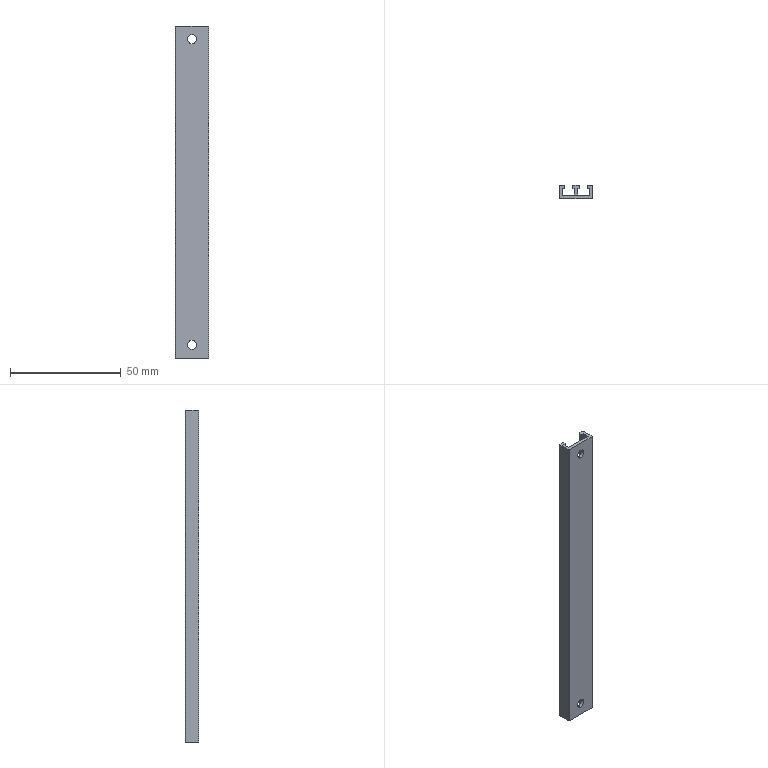Part | STEP file | 06-04 sensor mounting strip | 1 solid | 39 faces | box 15 x 6 x 150 mm | volume 6689 mm3 | plane 23 | cylinder 16 | commonest cylinder face diameters 0.4 x12 4 x4
STEP:
#1=CARTESIAN_POINT('',(7.5,0.,-146.));
#2=VERTEX_POINT('',#1);
#3=CARTESIAN_POINT('',(7.5,0.,-142.));
#4=VERTEX_POINT('',#3);
#5=CARTESIAN_POINT('',(7.5,0.,-144.));
#6=DIRECTION('',(0.,1.,0.));
#7=DIRECTION('',(0.,0.,-1.));
#8=AXIS2_PLACEMENT_3D('',#5,#6,#7);
#9=CIRCLE('',#8,2.);
#10=EDGE_CURVE('',#2,#4,#9,.T.);
#11=ORIENTED_EDGE('',*,*,#10,.F.);
#12=CARTESIAN_POINT('',(7.5,1.5,-146.));
#13=VERTEX_POINT('',#12);
#14=CARTESIAN_POINT('',(7.5,0.,-146.));
#15=DIRECTION('',(0.,1.,0.));
#16=VECTOR('',#15,1000.);
#17=LINE('',#14,#16);
#18=EDGE_CURVE('',#2,#13,#17,.T.);
#19=ORIENTED_EDGE('',*,*,#18,.T.);
#20=CARTESIAN_POINT('',(7.5,1.5,-142.));
#21=VERTEX_POINT('',#20);
#22=CARTESIAN_POINT('',(7.5,1.5,-144.));
#23=DIRECTION('',(0.,1.,0.));
#24=DIRECTION('',(0.,0.,-1.));
#25=AXIS2_PLACEMENT_3D('',#22,#23,#24);
#26=CIRCLE('',#25,2.);
#27=EDGE_CURVE('',#13,#21,#26,.T.);
#28=ORIENTED_EDGE('',*,*,#27,.T.);
#29=CARTESIAN_POINT('',(7.5,0.,-142.));
#30=DIRECTION('',(0.,1.,0.));
#31=VECTOR('',#30,1000.);
#32=LINE('',#29,#31);
#33=EDGE_CURVE('',#4,#21,#32,.T.);
#34=ORIENTED_EDGE('',*,*,#33,.F.);
#35=EDGE_LOOP('',(#11,#19,#28,#34));
#36=FACE_OUTER_BOUND('',#35,.T.);
#37=CARTESIAN_POINT('',(7.5,0.,-144.));
#38=DIRECTION('',(0.,1.,0.));
#39=DIRECTION('',(0.,0.,1.));
#40=AXIS2_PLACEMENT_3D('',#37,#38,#39);
#41=CYLINDRICAL_SURFACE('',#40,2.);
#42=ADVANCED_FACE('',(#36),#41,.F.);
#43=CARTESIAN_POINT('',(7.5,0.,-8.));
#44=VERTEX_POINT('',#43);
#45=CARTESIAN_POINT('',(7.5,0.,-4.));
#46=VERTEX_POINT('',#45);
#47=CARTESIAN_POINT('',(7.5,0.,-6.));
#48=DIRECTION('',(0.,1.,0.));
#49=DIRECTION('',(0.,0.,1.));
#50=AXIS2_PLACEMENT_3D('',#47,#48,#49);
#51=CIRCLE('',#50,2.);
#52=EDGE_CURVE('',#44,#46,#51,.T.);
#53=ORIENTED_EDGE('',*,*,#52,.F.);
#54=CARTESIAN_POINT('',(7.5,1.5,-8.));
#55=VERTEX_POINT('',#54);
#56=CARTESIAN_POINT('',(7.5,0.,-8.));
#57=DIRECTION('',(0.,1.,0.));
#58=VECTOR('',#57,1000.);
#59=LINE('',#56,#58);
#60=EDGE_CURVE('',#44,#55,#59,.T.);
#61=ORIENTED_EDGE('',*,*,#60,.T.);
#62=CARTESIAN_POINT('',(7.5,1.5,-4.));
#63=VERTEX_POINT('',#62);
#64=CARTESIAN_POINT('',(7.5,1.5,-6.));
#65=DIRECTION('',(0.,1.,0.));
#66=DIRECTION('',(0.,0.,1.));
#67=AXIS2_PLACEMENT_3D('',#64,#65,#66);
#68=CIRCLE('',#67,2.);
#69=EDGE_CURVE('',#55,#63,#68,.T.);
#70=ORIENTED_EDGE('',*,*,#69,.T.);
#71=CARTESIAN_POINT('',(7.5,0.,-4.));
#72=DIRECTION('',(0.,1.,0.));
#73=VECTOR('',#72,1000.);
#74=LINE('',#71,#73);
#75=EDGE_CURVE('',#46,#63,#74,.T.);
#76=ORIENTED_EDGE('',*,*,#75,.F.);
#77=EDGE_LOOP('',(#53,#61,#70,#76));
#78=FACE_OUTER_BOUND('',#77,.T.);
#79=CARTESIAN_POINT('',(7.5,0.,-6.));
#80=DIRECTION('',(0.,1.,0.));
#81=DIRECTION('',(0.,0.,1.));
#82=AXIS2_PLACEMENT_3D('',#79,#80,#81);
#83=CYLINDRICAL_SURFACE('',#82,2.);
#84=ADVANCED_FACE('',(#78),#83,.F.);
#85=CARTESIAN_POINT('',(1.25,1.5,-150.));
#86=VERTEX_POINT('',#85);
#87=CARTESIAN_POINT('',(1.25,4.5,-150.));
#88=VERTEX_POINT('',#87);
#89=CARTESIAN_POINT('',(1.25,4.5,-150.));
#90=DIRECTION('',(0.,1.,0.));
#91=VECTOR('',#90,1000.);
#92=LINE('',#89,#91);
#93=EDGE_CURVE('',#86,#88,#92,.T.);
#94=ORIENTED_EDGE('',*,*,#93,.F.);
#95=CARTESIAN_POINT('',(13.75,1.5,-150.));
#96=VERTEX_POINT('',#95);
#97=CARTESIAN_POINT('',(8.25,1.5,-150.));
#98=DIRECTION('',(-1.,0.,0.));
#99=VECTOR('',#98,1000.);
#100=LINE('',#97,#99);
#101=EDGE_CURVE('',#96,#86,#100,.T.);
#102=ORIENTED_EDGE('',*,*,#101,.F.);
#103=CARTESIAN_POINT('',(13.75,4.5,-150.));
#104=VERTEX_POINT('',#103);
#105=CARTESIAN_POINT('',(13.75,4.5,-150.));
#106=DIRECTION('',(0.,-1.,0.));
#107=VECTOR('',#106,1000.);
#108=LINE('',#105,#107);
#109=EDGE_CURVE('',#104,#96,#108,.T.);
#110=ORIENTED_EDGE('',*,*,#109,.F.);
#111=CARTESIAN_POINT('',(12.95,4.5,-150.));
#112=VERTEX_POINT('',#111);
#113=CARTESIAN_POINT('',(12.75,4.5,-150.));
#114=DIRECTION('',(1.,0.,0.));
#115=VECTOR('',#114,1000.);
#116=LINE('',#113,#115);
#117=EDGE_CURVE('',#112,#104,#116,.T.);
#118=ORIENTED_EDGE('',*,*,#117,.F.);
#119=CARTESIAN_POINT('',(12.75,4.7,-150.));
#120=VERTEX_POINT('',#119);
#121=CARTESIAN_POINT('',(12.95,4.7,-150.));
#122=DIRECTION('',(0.,0.,-1.));
#123=DIRECTION('',(1.,0.,0.));
#124=AXIS2_PLACEMENT_3D('',#121,#122,#123);
#125=CIRCLE('',#124,0.2);
#126=EDGE_CURVE('',#112,#120,#125,.T.);
#127=ORIENTED_EDGE('',*,*,#126,.T.);
#128=CARTESIAN_POINT('',(12.75,5.8,-150.));
#129=VERTEX_POINT('',#128);
#130=CARTESIAN_POINT('',(12.75,6.,-150.));
#131=DIRECTION('',(0.,-1.,0.));
#132=VECTOR('',#131,1000.);
#133=LINE('',#130,#132);
#134=EDGE_CURVE('',#129,#120,#133,.T.);
#135=ORIENTED_EDGE('',*,*,#134,.F.);
#136=CARTESIAN_POINT('',(12.95,6.,-150.));
#137=VERTEX_POINT('',#136);
#138=CARTESIAN_POINT('',(12.95,5.8,-150.));
#139=DIRECTION('',(0.,0.,-1.));
#140=DIRECTION('',(1.,0.,0.));
#141=AXIS2_PLACEMENT_3D('',#138,#139,#140);
#142=CIRCLE('',#141,0.2);
#143=EDGE_CURVE('',#129,#137,#142,.T.);
#144=ORIENTED_EDGE('',*,*,#143,.T.);
#145=CARTESIAN_POINT('',(14.8,6.,-150.));
#146=VERTEX_POINT('',#145);
#147=CARTESIAN_POINT('',(15.,6.,-150.));
#148=DIRECTION('',(-1.,0.,0.));
#149=VECTOR('',#148,1000.);
#150=LINE('',#147,#149);
#151=EDGE_CURVE('',#146,#137,#150,.T.);
#152=ORIENTED_EDGE('',*,*,#151,.F.);
#153=CARTESIAN_POINT('',(15.,5.8,-150.));
#154=VERTEX_POINT('',#153);
#155=CARTESIAN_POINT('',(14.8,5.8,-150.));
#156=DIRECTION('',(0.,0.,-1.));
#157=DIRECTION('',(1.,0.,0.));
#158=AXIS2_PLACEMENT_3D('',#155,#156,#157);
#159=CIRCLE('',#158,0.2);
#160=EDGE_CURVE('',#146,#154,#159,.T.);
#161=ORIENTED_EDGE('',*,*,#160,.T.);
#162=CARTESIAN_POINT('',(15.,0.2,-150.));
#163=VERTEX_POINT('',#162);
#164=CARTESIAN_POINT('',(15.,6.,-150.));
#165=DIRECTION('',(0.,1.,0.));
#166=VECTOR('',#165,1000.);
#167=LINE('',#164,#166);
#168=EDGE_CURVE('',#163,#154,#167,.T.);
#169=ORIENTED_EDGE('',*,*,#168,.F.);
#170=CARTESIAN_POINT('',(14.8,0.,-150.));
#171=VERTEX_POINT('',#170);
#172=CARTESIAN_POINT('',(14.8,0.2,-150.));
#173=DIRECTION('',(0.,0.,-1.));
#174=DIRECTION('',(1.,0.,0.));
#175=AXIS2_PLACEMENT_3D('',#172,#173,#174);
#176=CIRCLE('',#175,0.2);
#177=EDGE_CURVE('',#163,#171,#176,.T.);
#178=ORIENTED_EDGE('',*,*,#177,.T.);
#179=CARTESIAN_POINT('',(0.2,0.,-150.));
#180=VERTEX_POINT('',#179);
#181=CARTESIAN_POINT('',(0.,0.,-150.));
#182=DIRECTION('',(1.,0.,0.));
#183=VECTOR('',#182,1000.);
#184=LINE('',#181,#183);
#185=EDGE_CURVE('',#180,#171,#184,.T.);
#186=ORIENTED_EDGE('',*,*,#185,.F.);
#187=CARTESIAN_POINT('',(0.,0.2,-150.));
#188=VERTEX_POINT('',#187);
#189=CARTESIAN_POINT('',(0.2,0.2,-150.));
#190=DIRECTION('',(0.,0.,-1.));
#191=DIRECTION('',(1.,0.,0.));
#192=AXIS2_PLACEMENT_3D('',#189,#190,#191);
#193=CIRCLE('',#192,0.2);
#194=EDGE_CURVE('',#180,#188,#193,.T.);
#195=ORIENTED_EDGE('',*,*,#194,.T.);
#196=CARTESIAN_POINT('',(0.,5.8,-150.));
#197=VERTEX_POINT('',#196);
#198=CARTESIAN_POINT('',(0.,6.,-150.));
#199=DIRECTION('',(0.,-1.,0.));
#200=VECTOR('',#199,1000.);
#201=LINE('',#198,#200);
#202=EDGE_CURVE('',#197,#188,#201,.T.);
#203=ORIENTED_EDGE('',*,*,#202,.F.);
#204=CARTESIAN_POINT('',(0.2,6.,-150.));
#205=VERTEX_POINT('',#204);
#206=CARTESIAN_POINT('',(0.2,5.8,-150.));
#207=DIRECTION('',(0.,0.,-1.));
#208=DIRECTION('',(1.,0.,0.));
#209=AXIS2_PLACEMENT_3D('',#206,#207,#208);
#210=CIRCLE('',#209,0.2);
#211=EDGE_CURVE('',#197,#205,#210,.T.);
#212=ORIENTED_EDGE('',*,*,#211,.T.);
#213=CARTESIAN_POINT('',(2.05,6.,-150.));
#214=VERTEX_POINT('',#213);
#215=CARTESIAN_POINT('',(2.25,6.,-150.));
#216=DIRECTION('',(-1.,0.,0.));
#217=VECTOR('',#216,1000.);
#218=LINE('',#215,#217);
#219=EDGE_CURVE('',#214,#205,#218,.T.);
#220=ORIENTED_EDGE('',*,*,#219,.F.);
#221=CARTESIAN_POINT('',(2.25,5.8,-150.));
#222=VERTEX_POINT('',#221);
#223=CARTESIAN_POINT('',(2.05,5.8,-150.));
#224=DIRECTION('',(0.,0.,-1.));
#225=DIRECTION('',(1.,0.,0.));
#226=AXIS2_PLACEMENT_3D('',#223,#224,#225);
#227=CIRCLE('',#226,0.2);
#228=EDGE_CURVE('',#214,#222,#227,.T.);
#229=ORIENTED_EDGE('',*,*,#228,.T.);
#230=CARTESIAN_POINT('',(2.25,4.7,-150.));
#231=VERTEX_POINT('',#230);
#232=CARTESIAN_POINT('',(2.25,6.,-150.));
#233=DIRECTION('',(0.,1.,0.));
#234=VECTOR('',#233,1000.);
#235=LINE('',#232,#234);
#236=EDGE_CURVE('',#231,#222,#235,.T.);
#237=ORIENTED_EDGE('',*,*,#236,.F.);
#238=CARTESIAN_POINT('',(2.05,4.5,-150.));
#239=VERTEX_POINT('',#238);
#240=CARTESIAN_POINT('',(2.05,4.7,-150.));
#241=DIRECTION('',(0.,0.,-1.));
#242=DIRECTION('',(1.,0.,0.));
#243=AXIS2_PLACEMENT_3D('',#240,#241,#242);
#244=CIRCLE('',#243,0.2);
#245=EDGE_CURVE('',#231,#239,#244,.T.);
#246=ORIENTED_EDGE('',*,*,#245,.T.);
#247=CARTESIAN_POINT('',(1.25,4.5,-150.));
#248=DIRECTION('',(1.,0.,0.));
#249=VECTOR('',#248,1000.);
#250=LINE('',#247,#249);
#251=EDGE_CURVE('',#88,#239,#250,.T.);
#252=ORIENTED_EDGE('',*,*,#251,.F.);
#253=EDGE_LOOP('',(#94,#102,#110,#118,#127,#135,#144,#152,#161,#169,#178,#186,#195,#203,#212,#220,#229,#237,#246,#252));
#254=FACE_OUTER_BOUND('',#253,.T.);
#255=CARTESIAN_POINT('',(0.,0.,-150.));
#256=DIRECTION('',(0.,0.,1.));
#257=DIRECTION('',(1.,0.,0.));
#258=AXIS2_PLACEMENT_3D('',#255,#256,#257);
#259=PLANE('',#258);
#260=ADVANCED_FACE('',(#254),#259,.F.);
#261=CARTESIAN_POINT('',(13.75,4.5,0.));
#262=VERTEX_POINT('',#261);
#263=CARTESIAN_POINT('',(13.75,1.5,0.));
#264=VERTEX_POINT('',#263);
#265=CARTESIAN_POINT('',(13.75,4.5,0.));
#266=DIRECTION('',(0.,-1.,0.));
#267=VECTOR('',#266,1000.);
#268=LINE('',#265,#267);
#269=EDGE_CURVE('',#262,#264,#268,.T.);
#270=ORIENTED_EDGE('',*,*,#269,.T.);
#271=CARTESIAN_POINT('',(1.25,1.5,0.));
#272=VERTEX_POINT('',#271);
#273=CARTESIAN_POINT('',(1.25,1.5,0.));
#274=DIRECTION('',(-1.,0.,0.));
#275=VECTOR('',#274,1000.);
#276=LINE('',#273,#275);
#277=EDGE_CURVE('',#264,#272,#276,.T.);
#278=ORIENTED_EDGE('',*,*,#277,.T.);
#279=CARTESIAN_POINT('',(1.25,4.5,0.));
#280=VERTEX_POINT('',#279);
#281=CARTESIAN_POINT('',(1.25,4.5,0.));
#282=DIRECTION('',(0.,1.,0.));
#283=VECTOR('',#282,1000.);
#284=LINE('',#281,#283);
#285=EDGE_CURVE('',#272,#280,#284,.T.);
#286=ORIENTED_EDGE('',*,*,#285,.T.);
#287=CARTESIAN_POINT('',(2.05,4.5,0.));
#288=VERTEX_POINT('',#287);
#289=CARTESIAN_POINT('',(1.25,4.5,0.));
#290=DIRECTION('',(1.,0.,0.));
#291=VECTOR('',#290,1000.);
#292=LINE('',#289,#291);
#293=EDGE_CURVE('',#280,#288,#292,.T.);
#294=ORIENTED_EDGE('',*,*,#293,.T.);
#295=CARTESIAN_POINT('',(2.25,4.7,0.));
#296=VERTEX_POINT('',#295);
#297=CARTESIAN_POINT('',(2.05,4.7,0.));
#298=DIRECTION('',(0.,0.,1.));
#299=DIRECTION('',(1.,0.,0.));
#300=AXIS2_PLACEMENT_3D('',#297,#298,#299);
#301=CIRCLE('',#300,0.2);
#302=EDGE_CURVE('',#288,#296,#301,.T.);
#303=ORIENTED_EDGE('',*,*,#302,.T.);
#304=CARTESIAN_POINT('',(2.25,5.8,0.));
#305=VERTEX_POINT('',#304);
#306=CARTESIAN_POINT('',(2.25,6.,0.));
#307=DIRECTION('',(0.,1.,0.));
#308=VECTOR('',#307,1000.);
#309=LINE('',#306,#308);
#310=EDGE_CURVE('',#296,#305,#309,.T.);
#311=ORIENTED_EDGE('',*,*,#310,.T.);
#312=CARTESIAN_POINT('',(2.05,6.,0.));
#313=VERTEX_POINT('',#312);
#314=CARTESIAN_POINT('',(2.05,5.8,0.));
#315=DIRECTION('',(0.,0.,1.));
#316=DIRECTION('',(1.,0.,0.));
#317=AXIS2_PLACEMENT_3D('',#314,#315,#316);
#318=CIRCLE('',#317,0.2);
#319=EDGE_CURVE('',#305,#313,#318,.T.);
#320=ORIENTED_EDGE('',*,*,#319,.T.);
#321=CARTESIAN_POINT('',(0.2,6.,0.));
#322=VERTEX_POINT('',#321);
#323=CARTESIAN_POINT('',(2.25,6.,0.));
#324=DIRECTION('',(-1.,0.,0.));
#325=VECTOR('',#324,1000.);
#326=LINE('',#323,#325);
#327=EDGE_CURVE('',#313,#322,#326,.T.);
#328=ORIENTED_EDGE('',*,*,#327,.T.);
#329=CARTESIAN_POINT('',(0.,5.8,0.));
#330=VERTEX_POINT('',#329);
#331=CARTESIAN_POINT('',(0.2,5.8,0.));
#332=DIRECTION('',(0.,0.,1.));
#333=DIRECTION('',(1.,0.,0.));
#334=AXIS2_PLACEMENT_3D('',#331,#332,#333);
#335=CIRCLE('',#334,0.2);
#336=EDGE_CURVE('',#322,#330,#335,.T.);
#337=ORIENTED_EDGE('',*,*,#336,.T.);
#338=CARTESIAN_POINT('',(0.,0.2,0.));
#339=VERTEX_POINT('',#338);
#340=CARTESIAN_POINT('',(0.,6.,0.));
#341=DIRECTION('',(0.,-1.,0.));
#342=VECTOR('',#341,1000.);
#343=LINE('',#340,#342);
#344=EDGE_CURVE('',#330,#339,#343,.T.);
#345=ORIENTED_EDGE('',*,*,#344,.T.);
#346=CARTESIAN_POINT('',(0.2,0.,0.));
#347=VERTEX_POINT('',#346);
#348=CARTESIAN_POINT('',(0.2,0.2,0.));
#349=DIRECTION('',(0.,0.,1.));
#350=DIRECTION('',(1.,0.,0.));
#351=AXIS2_PLACEMENT_3D('',#348,#349,#350);
#352=CIRCLE('',#351,0.2);
#353=EDGE_CURVE('',#339,#347,#352,.T.);
#354=ORIENTED_EDGE('',*,*,#353,.T.);
#355=CARTESIAN_POINT('',(14.8,0.,0.));
#356=VERTEX_POINT('',#355);
#357=CARTESIAN_POINT('',(0.,0.,0.));
#358=DIRECTION('',(1.,0.,0.));
#359=VECTOR('',#358,1000.);
#360=LINE('',#357,#359);
#361=EDGE_CURVE('',#347,#356,#360,.T.);
#362=ORIENTED_EDGE('',*,*,#361,.T.);
#363=CARTESIAN_POINT('',(15.,0.2,0.));
#364=VERTEX_POINT('',#363);
#365=CARTESIAN_POINT('',(14.8,0.2,0.));
#366=DIRECTION('',(0.,0.,1.));
#367=DIRECTION('',(1.,0.,0.));
#368=AXIS2_PLACEMENT_3D('',#365,#366,#367);
#369=CIRCLE('',#368,0.2);
#370=EDGE_CURVE('',#356,#364,#369,.T.);
#371=ORIENTED_EDGE('',*,*,#370,.T.);
#372=CARTESIAN_POINT('',(15.,5.8,0.));
#373=VERTEX_POINT('',#372);
#374=CARTESIAN_POINT('',(15.,6.,0.));
#375=DIRECTION('',(0.,1.,0.));
#376=VECTOR('',#375,1000.);
#377=LINE('',#374,#376);
#378=EDGE_CURVE('',#364,#373,#377,.T.);
#379=ORIENTED_EDGE('',*,*,#378,.T.);
#380=CARTESIAN_POINT('',(14.8,6.,0.));
#381=VERTEX_POINT('',#380);
#382=CARTESIAN_POINT('',(14.8,5.8,0.));
#383=DIRECTION('',(0.,0.,1.));
#384=DIRECTION('',(1.,0.,0.));
#385=AXIS2_PLACEMENT_3D('',#382,#383,#384);
#386=CIRCLE('',#385,0.2);
#387=EDGE_CURVE('',#373,#381,#386,.T.);
#388=ORIENTED_EDGE('',*,*,#387,.T.);
#389=CARTESIAN_POINT('',(12.95,6.,0.));
#390=VERTEX_POINT('',#389);
#391=CARTESIAN_POINT('',(15.,6.,0.));
#392=DIRECTION('',(-1.,0.,0.));
#393=VECTOR('',#392,1000.);
#394=LINE('',#391,#393);
#395=EDGE_CURVE('',#381,#390,#394,.T.);
#396=ORIENTED_EDGE('',*,*,#395,.T.);
#397=CARTESIAN_POINT('',(12.75,5.8,0.));
#398=VERTEX_POINT('',#397);
#399=CARTESIAN_POINT('',(12.95,5.8,0.));
#400=DIRECTION('',(0.,0.,1.));
#401=DIRECTION('',(1.,0.,0.));
#402=AXIS2_PLACEMENT_3D('',#399,#400,#401);
#403=CIRCLE('',#402,0.2);
#404=EDGE_CURVE('',#390,#398,#403,.T.);
#405=ORIENTED_EDGE('',*,*,#404,.T.);
#406=CARTESIAN_POINT('',(12.75,4.7,0.));
#407=VERTEX_POINT('',#406);
#408=CARTESIAN_POINT('',(12.75,6.,0.));
#409=DIRECTION('',(0.,-1.,0.));
#410=VECTOR('',#409,1000.);
#411=LINE('',#408,#410);
#412=EDGE_CURVE('',#398,#407,#411,.T.);
#413=ORIENTED_EDGE('',*,*,#412,.T.);
#414=CARTESIAN_POINT('',(12.95,4.5,0.));
#415=VERTEX_POINT('',#414);
#416=CARTESIAN_POINT('',(12.95,4.7,0.));
#417=DIRECTION('',(0.,0.,1.));
#418=DIRECTION('',(1.,0.,0.));
#419=AXIS2_PLACEMENT_3D('',#416,#417,#418);
#420=CIRCLE('',#419,0.2);
#421=EDGE_CURVE('',#407,#415,#420,.T.);
#422=ORIENTED_EDGE('',*,*,#421,.T.);
#423=CARTESIAN_POINT('',(12.75,4.5,0.));
#424=DIRECTION('',(1.,0.,0.));
#425=VECTOR('',#424,1000.);
#426=LINE('',#423,#425);
#427=EDGE_CURVE('',#415,#262,#426,.T.);
#428=ORIENTED_EDGE('',*,*,#427,.T.);
#429=EDGE_LOOP('',(#270,#278,#286,#294,#303,#311,#320,#328,#337,#345,#354,#362,#371,#379,#388,#396,#405,#413,#422,#428));
#430=FACE_OUTER_BOUND('',#429,.T.);
#431=CARTESIAN_POINT('',(0.,0.,0.));
#432=DIRECTION('',(0.,0.,1.));
#433=DIRECTION('',(1.,0.,0.));
#434=AXIS2_PLACEMENT_3D('',#431,#432,#433);
#435=PLANE('',#434);
#436=ADVANCED_FACE('',(#430),#435,.T.);
#437=ORIENTED_EDGE('',*,*,#202,.T.);
#438=CARTESIAN_POINT('',(0.,0.2,-150.));
#439=DIRECTION('',(0.,0.,1.));
#440=VECTOR('',#439,1000.);
#441=LINE('',#438,#440);
#442=EDGE_CURVE('',#188,#339,#441,.T.);
#443=ORIENTED_EDGE('',*,*,#442,.T.);
#444=ORIENTED_EDGE('',*,*,#344,.F.);
#445=CARTESIAN_POINT('',(0.,5.8,-150.));
#446=DIRECTION('',(0.,0.,-1.));
#447=VECTOR('',#446,1000.);
#448=LINE('',#445,#447);
#449=EDGE_CURVE('',#330,#197,#448,.T.);
#450=ORIENTED_EDGE('',*,*,#449,.T.);
#451=EDGE_LOOP('',(#437,#443,#444,#450));
#452=FACE_OUTER_BOUND('',#451,.T.);
#453=CARTESIAN_POINT('',(0.,6.,-150.));
#454=DIRECTION('',(-1.,0.,0.));
#455=DIRECTION('',(0.,0.,1.));
#456=AXIS2_PLACEMENT_3D('',#453,#454,#455);
#457=PLANE('',#456);
#458=ADVANCED_FACE('',(#452),#457,.T.);
#459=ORIENTED_EDGE('',*,*,#327,.F.);
#460=CARTESIAN_POINT('',(2.05,6.,-150.));
#461=DIRECTION('',(0.,0.,-1.));
#462=VECTOR('',#461,1000.);
#463=LINE('',#460,#462);
#464=EDGE_CURVE('',#313,#214,#463,.T.);
#465=ORIENTED_EDGE('',*,*,#464,.T.);
#466=ORIENTED_EDGE('',*,*,#219,.T.);
#467=CARTESIAN_POINT('',(0.2,6.,-150.));
#468=DIRECTION('',(0.,0.,1.));
#469=VECTOR('',#468,1000.);
#470=LINE('',#467,#469);
#471=EDGE_CURVE('',#205,#322,#470,.T.);
#472=ORIENTED_EDGE('',*,*,#471,.T.);
#473=EDGE_LOOP('',(#459,#465,#466,#472));
#474=FACE_OUTER_BOUND('',#473,.T.);
#475=CARTESIAN_POINT('',(2.25,6.,-150.));
#476=DIRECTION('',(0.,1.,0.));
#477=DIRECTION('',(0.,0.,1.));
#478=AXIS2_PLACEMENT_3D('',#475,#476,#477);
#479=PLANE('',#478);
#480=ADVANCED_FACE('',(#474),#479,.T.);
#481=ORIENTED_EDGE('',*,*,#310,.F.);
#482=CARTESIAN_POINT('',(2.25,4.7,-150.));
#483=DIRECTION('',(0.,0.,-1.));
#484=VECTOR('',#483,1000.);
#485=LINE('',#482,#484);
#486=EDGE_CURVE('',#296,#231,#485,.T.);
#487=ORIENTED_EDGE('',*,*,#486,.T.);
#488=ORIENTED_EDGE('',*,*,#236,.T.);
#489=CARTESIAN_POINT('',(2.25,5.8,-150.));
#490=DIRECTION('',(0.,0.,1.));
#491=VECTOR('',#490,1000.);
#492=LINE('',#489,#491);
#493=EDGE_CURVE('',#222,#305,#492,.T.);
#494=ORIENTED_EDGE('',*,*,#493,.T.);
#495=EDGE_LOOP('',(#481,#487,#488,#494));
#496=FACE_OUTER_BOUND('',#495,.T.);
#497=CARTESIAN_POINT('',(2.25,6.,-150.));
#498=DIRECTION('',(1.,0.,0.));
#499=DIRECTION('',(0.,0.,-1.));
#500=AXIS2_PLACEMENT_3D('',#497,#498,#499);
#501=PLANE('',#500);
#502=ADVANCED_FACE('',(#496),#501,.T.);
#503=ORIENTED_EDGE('',*,*,#251,.T.);
#504=CARTESIAN_POINT('',(2.05,4.5,-150.));
#505=DIRECTION('',(0.,0.,1.));
#506=VECTOR('',#505,1000.);
#507=LINE('',#504,#506);
#508=EDGE_CURVE('',#239,#288,#507,.T.);
#509=ORIENTED_EDGE('',*,*,#508,.T.);
#510=ORIENTED_EDGE('',*,*,#293,.F.);
#511=CARTESIAN_POINT('',(1.25,4.5,-150.));
#512=DIRECTION('',(0.,0.,1.));
#513=VECTOR('',#512,1000.);
#514=LINE('',#511,#513);
#515=EDGE_CURVE('',#88,#280,#514,.T.);
#516=ORIENTED_EDGE('',*,*,#515,.F.);
#517=EDGE_LOOP('',(#503,#509,#510,#516));
#518=FACE_OUTER_BOUND('',#517,.T.);
#519=CARTESIAN_POINT('',(1.25,4.5,-150.));
#520=DIRECTION('',(0.,-1.,0.));
#521=DIRECTION('',(0.,0.,-1.));
#522=AXIS2_PLACEMENT_3D('',#519,#520,#521);
#523=PLANE('',#522);
#524=ADVANCED_FACE('',(#518),#523,.T.);
#525=ORIENTED_EDGE('',*,*,#285,.F.);
#526=CARTESIAN_POINT('',(1.25,1.5,-150.));
#527=DIRECTION('',(0.,0.,1.));
#528=VECTOR('',#527,1000.);
#529=LINE('',#526,#528);
#530=EDGE_CURVE('',#86,#272,#529,.T.);
#531=ORIENTED_EDGE('',*,*,#530,.F.);
#532=ORIENTED_EDGE('',*,*,#93,.T.);
#533=ORIENTED_EDGE('',*,*,#515,.T.);
#534=EDGE_LOOP('',(#525,#531,#532,#533));
#535=FACE_OUTER_BOUND('',#534,.T.);
#536=CARTESIAN_POINT('',(1.25,4.5,-150.));
#537=DIRECTION('',(1.,0.,0.));
#538=DIRECTION('',(0.,0.,-1.));
#539=AXIS2_PLACEMENT_3D('',#536,#537,#538);
#540=PLANE('',#539);
#541=ADVANCED_FACE('',(#535),#540,.T.);
#542=CARTESIAN_POINT('',(7.5,1.5,-144.));
#543=DIRECTION('',(0.,1.,0.));
#544=DIRECTION('',(0.,0.,-1.));
#545=AXIS2_PLACEMENT_3D('',#542,#543,#544);
#546=CIRCLE('',#545,2.);
#547=EDGE_CURVE('',#21,#13,#546,.T.);
#548=ORIENTED_EDGE('',*,*,#547,.F.);
#549=ORIENTED_EDGE('',*,*,#27,.F.);
#550=EDGE_LOOP('',(#548,#549));
#551=FACE_BOUND('',#550,.T.);
#552=CARTESIAN_POINT('',(7.5,1.5,-6.));
#553=DIRECTION('',(0.,1.,0.));
#554=DIRECTION('',(0.,0.,1.));
#555=AXIS2_PLACEMENT_3D('',#552,#553,#554);
#556=CIRCLE('',#555,2.);
#557=EDGE_CURVE('',#63,#55,#556,.T.);
#558=ORIENTED_EDGE('',*,*,#557,.F.);
#559=ORIENTED_EDGE('',*,*,#69,.F.);
#560=EDGE_LOOP('',(#558,#559));
#561=FACE_BOUND('',#560,.T.);
#562=ORIENTED_EDGE('',*,*,#101,.T.);
#563=ORIENTED_EDGE('',*,*,#530,.T.);
#564=ORIENTED_EDGE('',*,*,#277,.F.);
#565=CARTESIAN_POINT('',(13.75,1.5,-150.));
#566=DIRECTION('',(0.,0.,1.));
#567=VECTOR('',#566,1000.);
#568=LINE('',#565,#567);
#569=EDGE_CURVE('',#96,#264,#568,.T.);
#570=ORIENTED_EDGE('',*,*,#569,.F.);
#571=EDGE_LOOP('',(#562,#563,#564,#570));
#572=FACE_OUTER_BOUND('',#571,.T.);
#573=CARTESIAN_POINT('',(6.75,1.5,-138.));
#574=VERTEX_POINT('',#573);
#575=CARTESIAN_POINT('',(6.75,1.5,-12.));
#576=VERTEX_POINT('',#575);
#577=CARTESIAN_POINT('',(6.75,1.5,-150.));
#578=DIRECTION('',(0.,0.,1.));
#579=VECTOR('',#578,1000.);
#580=LINE('',#577,#579);
#581=EDGE_CURVE('',#574,#576,#580,.T.);
#582=ORIENTED_EDGE('',*,*,#581,.F.);
#583=CARTESIAN_POINT('',(8.25,1.5,-138.));
#584=VERTEX_POINT('',#583);
#585=CARTESIAN_POINT('',(4.,1.5,-138.));
#586=DIRECTION('',(-1.,0.,0.));
#587=VECTOR('',#586,1000.);
#588=LINE('',#585,#587);
#589=EDGE_CURVE('',#584,#574,#588,.T.);
#590=ORIENTED_EDGE('',*,*,#589,.F.);
#591=CARTESIAN_POINT('',(8.25,1.5,-12.));
#592=VERTEX_POINT('',#591);
#593=CARTESIAN_POINT('',(8.25,1.5,-150.));
#594=DIRECTION('',(0.,0.,1.));
#595=VECTOR('',#594,1000.);
#596=LINE('',#593,#595);
#597=EDGE_CURVE('',#584,#592,#596,.T.);
#598=ORIENTED_EDGE('',*,*,#597,.T.);
#599=CARTESIAN_POINT('',(4.,1.5,-12.));
#600=DIRECTION('',(1.,0.,0.));
#601=VECTOR('',#600,1000.);
#602=LINE('',#599,#601);
#603=EDGE_CURVE('',#576,#592,#602,.T.);
#604=ORIENTED_EDGE('',*,*,#603,.F.);
#605=EDGE_LOOP('',(#582,#590,#598,#604));
#606=FACE_BOUND('',#605,.T.);
#607=CARTESIAN_POINT('',(1.25,1.5,-150.));
#608=DIRECTION('',(0.,1.,0.));
#609=DIRECTION('',(0.,0.,1.));
#610=AXIS2_PLACEMENT_3D('',#607,#608,#609);
#611=PLANE('',#610);
#612=ADVANCED_FACE('',(#551,#561,#572,#606),#611,.T.);
#613=CARTESIAN_POINT('',(6.75,4.5,-138.));
#614=VERTEX_POINT('',#613);
#615=CARTESIAN_POINT('',(6.75,4.5,-138.));
#616=DIRECTION('',(0.,1.,0.));
#617=VECTOR('',#616,1000.);
#618=LINE('',#615,#617);
#619=EDGE_CURVE('',#574,#614,#618,.T.);
#620=ORIENTED_EDGE('',*,*,#619,.F.);
#621=ORIENTED_EDGE('',*,*,#581,.T.);
#622=CARTESIAN_POINT('',(6.75,4.5,-12.));
#623=VERTEX_POINT('',#622);
#624=CARTESIAN_POINT('',(6.75,4.5,-12.));
#625=DIRECTION('',(0.,-1.,0.));
#626=VECTOR('',#625,1000.);
#627=LINE('',#624,#626);
#628=EDGE_CURVE('',#623,#576,#627,.T.);
#629=ORIENTED_EDGE('',*,*,#628,.F.);
#630=CARTESIAN_POINT('',(6.75,4.5,-150.));
#631=DIRECTION('',(0.,0.,1.));
#632=VECTOR('',#631,1000.);
#633=LINE('',#630,#632);
#634=EDGE_CURVE('',#614,#623,#633,.T.);
#635=ORIENTED_EDGE('',*,*,#634,.F.);
#636=EDGE_LOOP('',(#620,#621,#629,#635));
#637=FACE_OUTER_BOUND('',#636,.T.);
#638=CARTESIAN_POINT('',(6.75,4.5,-150.));
#639=DIRECTION('',(-1.,0.,0.));
#640=DIRECTION('',(0.,-1.,0.));
#641=AXIS2_PLACEMENT_3D('',#638,#639,#640);
#642=PLANE('',#641);
#643=ADVANCED_FACE('',(#637),#642,.T.);
#644=CARTESIAN_POINT('',(5.95,4.5,-138.));
#645=VERTEX_POINT('',#644);
#646=CARTESIAN_POINT('',(5.75,4.5,-138.));
#647=DIRECTION('',(-1.,0.,0.));
#648=VECTOR('',#647,1000.);
#649=LINE('',#646,#648);
#650=EDGE_CURVE('',#614,#645,#649,.T.);
#651=ORIENTED_EDGE('',*,*,#650,.F.);
#652=ORIENTED_EDGE('',*,*,#634,.T.);
#653=CARTESIAN_POINT('',(5.95,4.5,-12.));
#654=VERTEX_POINT('',#653);
#655=CARTESIAN_POINT('',(5.75,4.5,-12.));
#656=DIRECTION('',(1.,0.,0.));
#657=VECTOR('',#656,1000.);
#658=LINE('',#655,#657);
#659=EDGE_CURVE('',#654,#623,#658,.T.);
#660=ORIENTED_EDGE('',*,*,#659,.F.);
#661=CARTESIAN_POINT('',(5.95,4.5,-150.));
#662=DIRECTION('',(0.,0.,-1.));
#663=VECTOR('',#662,1000.);
#664=LINE('',#661,#663);
#665=EDGE_CURVE('',#654,#645,#664,.T.);
#666=ORIENTED_EDGE('',*,*,#665,.T.);
#667=EDGE_LOOP('',(#651,#652,#660,#666));
#668=FACE_OUTER_BOUND('',#667,.T.);
#669=CARTESIAN_POINT('',(5.75,4.5,-150.));
#670=DIRECTION('',(0.,-1.,0.));
#671=DIRECTION('',(0.,0.,-1.));
#672=AXIS2_PLACEMENT_3D('',#669,#670,#671);
#673=PLANE('',#672);
#674=ADVANCED_FACE('',(#668),#673,.T.);
#675=CARTESIAN_POINT('',(5.75,4.7,-138.));
#676=VERTEX_POINT('',#675);
#677=CARTESIAN_POINT('',(5.75,5.8,-138.));
#678=VERTEX_POINT('',#677);
#679=CARTESIAN_POINT('',(5.75,6.,-138.));
#680=DIRECTION('',(0.,1.,0.));
#681=VECTOR('',#680,1000.);
#682=LINE('',#679,#681);
#683=EDGE_CURVE('',#676,#678,#682,.T.);
#684=ORIENTED_EDGE('',*,*,#683,.F.);
#685=CARTESIAN_POINT('',(5.75,4.7,-12.));
#686=VERTEX_POINT('',#685);
#687=CARTESIAN_POINT('',(5.75,4.7,-150.));
#688=DIRECTION('',(0.,0.,1.));
#689=VECTOR('',#688,1000.);
#690=LINE('',#687,#689);
#691=EDGE_CURVE('',#676,#686,#690,.T.);
#692=ORIENTED_EDGE('',*,*,#691,.T.);
#693=CARTESIAN_POINT('',(5.75,5.8,-12.));
#694=VERTEX_POINT('',#693);
#695=CARTESIAN_POINT('',(5.75,6.,-12.));
#696=DIRECTION('',(0.,-1.,0.));
#697=VECTOR('',#696,1000.);
#698=LINE('',#695,#697);
#699=EDGE_CURVE('',#694,#686,#698,.T.);
#700=ORIENTED_EDGE('',*,*,#699,.F.);
#701=CARTESIAN_POINT('',(5.75,5.8,-150.));
#702=DIRECTION('',(0.,0.,-1.));
#703=VECTOR('',#702,1000.);
#704=LINE('',#701,#703);
#705=EDGE_CURVE('',#694,#678,#704,.T.);
#706=ORIENTED_EDGE('',*,*,#705,.T.);
#707=EDGE_LOOP('',(#684,#692,#700,#706));
#708=FACE_OUTER_BOUND('',#707,.T.);
#709=CARTESIAN_POINT('',(5.75,6.,-150.));
#710=DIRECTION('',(-1.,0.,0.));
#711=DIRECTION('',(0.,-1.,0.));
#712=AXIS2_PLACEMENT_3D('',#709,#710,#711);
#713=PLANE('',#712);
#714=ADVANCED_FACE('',(#708),#713,.T.);
#715=CARTESIAN_POINT('',(5.95,6.,-138.));
#716=VERTEX_POINT('',#715);
#717=CARTESIAN_POINT('',(9.05,6.,-138.));
#718=VERTEX_POINT('',#717);
#719=CARTESIAN_POINT('',(4.,6.,-138.));
#720=DIRECTION('',(1.,0.,0.));
#721=VECTOR('',#720,1000.);
#722=LINE('',#719,#721);
#723=EDGE_CURVE('',#716,#718,#722,.T.);
#724=ORIENTED_EDGE('',*,*,#723,.F.);
#725=CARTESIAN_POINT('',(5.95,6.,-12.));
#726=VERTEX_POINT('',#725);
#727=CARTESIAN_POINT('',(5.95,6.,-150.));
#728=DIRECTION('',(0.,0.,1.));
#729=VECTOR('',#728,1000.);
#730=LINE('',#727,#729);
#731=EDGE_CURVE('',#716,#726,#730,.T.);
#732=ORIENTED_EDGE('',*,*,#731,.T.);
#733=CARTESIAN_POINT('',(9.05,6.,-12.));
#734=VERTEX_POINT('',#733);
#735=CARTESIAN_POINT('',(4.,6.,-12.));
#736=DIRECTION('',(-1.,0.,0.));
#737=VECTOR('',#736,1000.);
#738=LINE('',#735,#737);
#739=EDGE_CURVE('',#734,#726,#738,.T.);
#740=ORIENTED_EDGE('',*,*,#739,.F.);
#741=CARTESIAN_POINT('',(9.05,6.,-150.));
#742=DIRECTION('',(0.,0.,-1.));
#743=VECTOR('',#742,1000.);
#744=LINE('',#741,#743);
#745=EDGE_CURVE('',#734,#718,#744,.T.);
#746=ORIENTED_EDGE('',*,*,#745,.T.);
#747=EDGE_LOOP('',(#724,#732,#740,#746));
#748=FACE_OUTER_BOUND('',#747,.T.);
#749=CARTESIAN_POINT('',(9.25,6.,-150.));
#750=DIRECTION('',(0.,1.,0.));
#751=DIRECTION('',(-1.,0.,0.));
#752=AXIS2_PLACEMENT_3D('',#749,#750,#751);
#753=PLANE('',#752);
#754=ADVANCED_FACE('',(#748),#753,.T.);
#755=CARTESIAN_POINT('',(9.25,5.8,-138.));
#756=VERTEX_POINT('',#755);
#757=CARTESIAN_POINT('',(9.25,4.7,-138.));
#758=VERTEX_POINT('',#757);
#759=CARTESIAN_POINT('',(9.25,6.,-138.));
#760=DIRECTION('',(0.,-1.,0.));
#761=VECTOR('',#760,1000.);
#762=LINE('',#759,#761);
#763=EDGE_CURVE('',#756,#758,#762,.T.);
#764=ORIENTED_EDGE('',*,*,#763,.F.);
#765=CARTESIAN_POINT('',(9.25,5.8,-12.));
#766=VERTEX_POINT('',#765);
#767=CARTESIAN_POINT('',(9.25,5.8,-150.));
#768=DIRECTION('',(0.,0.,1.));
#769=VECTOR('',#768,1000.);
#770=LINE('',#767,#769);
#771=EDGE_CURVE('',#756,#766,#770,.T.);
#772=ORIENTED_EDGE('',*,*,#771,.T.);
#773=CARTESIAN_POINT('',(9.25,4.7,-12.));
#774=VERTEX_POINT('',#773);
#775=CARTESIAN_POINT('',(9.25,6.,-12.));
#776=DIRECTION('',(0.,1.,0.));
#777=VECTOR('',#776,1000.);
#778=LINE('',#775,#777);
#779=EDGE_CURVE('',#774,#766,#778,.T.);
#780=ORIENTED_EDGE('',*,*,#779,.F.);
#781=CARTESIAN_POINT('',(9.25,4.7,-150.));
#782=DIRECTION('',(0.,0.,-1.));
#783=VECTOR('',#782,1000.);
#784=LINE('',#781,#783);
#785=EDGE_CURVE('',#774,#758,#784,.T.);
#786=ORIENTED_EDGE('',*,*,#785,.T.);
#787=EDGE_LOOP('',(#764,#772,#780,#786));
#788=FACE_OUTER_BOUND('',#787,.T.);
#789=CARTESIAN_POINT('',(9.25,6.,-150.));
#790=DIRECTION('',(1.,0.,0.));
#791=DIRECTION('',(0.,1.,0.));
#792=AXIS2_PLACEMENT_3D('',#789,#790,#791);
#793=PLANE('',#792);
#794=ADVANCED_FACE('',(#788),#793,.T.);
#795=CARTESIAN_POINT('',(9.05,4.5,-138.));
#796=VERTEX_POINT('',#795);
#797=CARTESIAN_POINT('',(8.25,4.5,-138.));
#798=VERTEX_POINT('',#797);
#799=CARTESIAN_POINT('',(8.25,4.5,-138.));
#800=DIRECTION('',(-1.,0.,0.));
#801=VECTOR('',#800,1000.);
#802=LINE('',#799,#801);
#803=EDGE_CURVE('',#796,#798,#802,.T.);
#804=ORIENTED_EDGE('',*,*,#803,.F.);
#805=CARTESIAN_POINT('',(9.05,4.5,-12.));
#806=VERTEX_POINT('',#805);
#807=CARTESIAN_POINT('',(9.05,4.5,-150.));
#808=DIRECTION('',(0.,0.,1.));
#809=VECTOR('',#808,1000.);
#810=LINE('',#807,#809);
#811=EDGE_CURVE('',#796,#806,#810,.T.);
#812=ORIENTED_EDGE('',*,*,#811,.T.);
#813=CARTESIAN_POINT('',(8.25,4.5,-12.));
#814=VERTEX_POINT('',#813);
#815=CARTESIAN_POINT('',(8.25,4.5,-12.));
#816=DIRECTION('',(1.,0.,0.));
#817=VECTOR('',#816,1000.);
#818=LINE('',#815,#817);
#819=EDGE_CURVE('',#814,#806,#818,.T.);
#820=ORIENTED_EDGE('',*,*,#819,.F.);
#821=CARTESIAN_POINT('',(8.25,4.5,-150.));
#822=DIRECTION('',(0.,0.,1.));
#823=VECTOR('',#822,1000.);
#824=LINE('',#821,#823);
#825=EDGE_CURVE('',#798,#814,#824,.T.);
#826=ORIENTED_EDGE('',*,*,#825,.F.);
#827=EDGE_LOOP('',(#804,#812,#820,#826));
#828=FACE_OUTER_BOUND('',#827,.T.);
#829=CARTESIAN_POINT('',(8.25,4.5,-150.));
#830=DIRECTION('',(0.,-1.,0.));
#831=DIRECTION('',(1.,0.,0.));
#832=AXIS2_PLACEMENT_3D('',#829,#830,#831);
#833=PLANE('',#832);
#834=ADVANCED_FACE('',(#828),#833,.T.);
#835=CARTESIAN_POINT('',(8.25,4.5,-138.));
#836=DIRECTION('',(0.,-1.,0.));
#837=VECTOR('',#836,1000.);
#838=LINE('',#835,#837);
#839=EDGE_CURVE('',#798,#584,#838,.T.);
#840=ORIENTED_EDGE('',*,*,#839,.F.);
#841=ORIENTED_EDGE('',*,*,#825,.T.);
#842=CARTESIAN_POINT('',(8.25,4.5,-12.));
#843=DIRECTION('',(0.,1.,0.));
#844=VECTOR('',#843,1000.);
#845=LINE('',#842,#844);
#846=EDGE_CURVE('',#592,#814,#845,.T.);
#847=ORIENTED_EDGE('',*,*,#846,.F.);
#848=ORIENTED_EDGE('',*,*,#597,.F.);
#849=EDGE_LOOP('',(#840,#841,#847,#848));
#850=FACE_OUTER_BOUND('',#849,.T.);
#851=CARTESIAN_POINT('',(8.25,4.5,-150.));
#852=DIRECTION('',(1.,0.,0.));
#853=DIRECTION('',(0.,1.,0.));
#854=AXIS2_PLACEMENT_3D('',#851,#852,#853);
#855=PLANE('',#854);
#856=ADVANCED_FACE('',(#850),#855,.T.);
#857=ORIENTED_EDGE('',*,*,#269,.F.);
#858=CARTESIAN_POINT('',(13.75,4.5,-150.));
#859=DIRECTION('',(0.,0.,1.));
#860=VECTOR('',#859,1000.);
#861=LINE('',#858,#860);
#862=EDGE_CURVE('',#104,#262,#861,.T.);
#863=ORIENTED_EDGE('',*,*,#862,.F.);
#864=ORIENTED_EDGE('',*,*,#109,.T.);
#865=ORIENTED_EDGE('',*,*,#569,.T.);
#866=EDGE_LOOP('',(#857,#863,#864,#865));
#867=FACE_OUTER_BOUND('',#866,.T.);
#868=CARTESIAN_POINT('',(13.75,4.5,-150.));
#869=DIRECTION('',(-1.,0.,0.));
#870=DIRECTION('',(0.,0.,1.));
#871=AXIS2_PLACEMENT_3D('',#868,#869,#870);
#872=PLANE('',#871);
#873=ADVANCED_FACE('',(#867),#872,.T.);
#874=ORIENTED_EDGE('',*,*,#427,.F.);
#875=CARTESIAN_POINT('',(12.95,4.5,-150.));
#876=DIRECTION('',(0.,0.,-1.));
#877=VECTOR('',#876,1000.);
#878=LINE('',#875,#877);
#879=EDGE_CURVE('',#415,#112,#878,.T.);
#880=ORIENTED_EDGE('',*,*,#879,.T.);
#881=ORIENTED_EDGE('',*,*,#117,.T.);
#882=ORIENTED_EDGE('',*,*,#862,.T.);
#883=EDGE_LOOP('',(#874,#880,#881,#882));
#884=FACE_OUTER_BOUND('',#883,.T.);
#885=CARTESIAN_POINT('',(12.75,4.5,-150.));
#886=DIRECTION('',(0.,-1.,0.));
#887=DIRECTION('',(1.,0.,0.));
#888=AXIS2_PLACEMENT_3D('',#885,#886,#887);
#889=PLANE('',#888);
#890=ADVANCED_FACE('',(#884),#889,.T.);
#891=ORIENTED_EDGE('',*,*,#134,.T.);
#892=CARTESIAN_POINT('',(12.75,4.7,-150.));
#893=DIRECTION('',(0.,0.,1.));
#894=VECTOR('',#893,1000.);
#895=LINE('',#892,#894);
#896=EDGE_CURVE('',#120,#407,#895,.T.);
#897=ORIENTED_EDGE('',*,*,#896,.T.);
#898=ORIENTED_EDGE('',*,*,#412,.F.);
#899=CARTESIAN_POINT('',(12.75,5.8,-150.));
#900=DIRECTION('',(0.,0.,-1.));
#901=VECTOR('',#900,1000.);
#902=LINE('',#899,#901);
#903=EDGE_CURVE('',#398,#129,#902,.T.);
#904=ORIENTED_EDGE('',*,*,#903,.T.);
#905=EDGE_LOOP('',(#891,#897,#898,#904));
#906=FACE_OUTER_BOUND('',#905,.T.);
#907=CARTESIAN_POINT('',(12.75,6.,-150.));
#908=DIRECTION('',(-1.,0.,0.));
#909=DIRECTION('',(0.,-1.,0.));
#910=AXIS2_PLACEMENT_3D('',#907,#908,#909);
#911=PLANE('',#910);
#912=ADVANCED_FACE('',(#906),#911,.T.);
#913=ORIENTED_EDGE('',*,*,#151,.T.);
#914=CARTESIAN_POINT('',(12.95,6.,-150.));
#915=DIRECTION('',(0.,0.,1.));
#916=VECTOR('',#915,1000.);
#917=LINE('',#914,#916);
#918=EDGE_CURVE('',#137,#390,#917,.T.);
#919=ORIENTED_EDGE('',*,*,#918,.T.);
#920=ORIENTED_EDGE('',*,*,#395,.F.);
#921=CARTESIAN_POINT('',(14.8,6.,-150.));
#922=DIRECTION('',(0.,0.,-1.));
#923=VECTOR('',#922,1000.);
#924=LINE('',#921,#923);
#925=EDGE_CURVE('',#381,#146,#924,.T.);
#926=ORIENTED_EDGE('',*,*,#925,.T.);
#927=EDGE_LOOP('',(#913,#919,#920,#926));
#928=FACE_OUTER_BOUND('',#927,.T.);
#929=CARTESIAN_POINT('',(15.,6.,-150.));
#930=DIRECTION('',(0.,1.,0.));
#931=DIRECTION('',(-1.,0.,0.));
#932=AXIS2_PLACEMENT_3D('',#929,#930,#931);
#933=PLANE('',#932);
#934=ADVANCED_FACE('',(#928),#933,.T.);
#935=ORIENTED_EDGE('',*,*,#378,.F.);
#936=CARTESIAN_POINT('',(15.,0.2,-150.));
#937=DIRECTION('',(0.,0.,-1.));
#938=VECTOR('',#937,1000.);
#939=LINE('',#936,#938);
#940=EDGE_CURVE('',#364,#163,#939,.T.);
#941=ORIENTED_EDGE('',*,*,#940,.T.);
#942=ORIENTED_EDGE('',*,*,#168,.T.);
#943=CARTESIAN_POINT('',(15.,5.8,-150.));
#944=DIRECTION('',(0.,0.,1.));
#945=VECTOR('',#944,1000.);
#946=LINE('',#943,#945);
#947=EDGE_CURVE('',#154,#373,#946,.T.);
#948=ORIENTED_EDGE('',*,*,#947,.T.);
#949=EDGE_LOOP('',(#935,#941,#942,#948));
#950=FACE_OUTER_BOUND('',#949,.T.);
#951=CARTESIAN_POINT('',(15.,6.,-150.));
#952=DIRECTION('',(1.,0.,0.));
#953=DIRECTION('',(0.,0.,-1.));
#954=AXIS2_PLACEMENT_3D('',#951,#952,#953);
#955=PLANE('',#954);
#956=ADVANCED_FACE('',(#950),#955,.T.);
#957=CARTESIAN_POINT('',(7.5,0.,-144.));
#958=DIRECTION('',(0.,1.,0.));
#959=DIRECTION('',(0.,0.,-1.));
#960=AXIS2_PLACEMENT_3D('',#957,#958,#959);
#961=CIRCLE('',#960,2.);
#962=EDGE_CURVE('',#4,#2,#961,.T.);
#963=ORIENTED_EDGE('',*,*,#962,.T.);
#964=ORIENTED_EDGE('',*,*,#10,.T.);
#965=EDGE_LOOP('',(#963,#964));
#966=FACE_BOUND('',#965,.T.);
#967=CARTESIAN_POINT('',(7.5,0.,-6.));
#968=DIRECTION('',(0.,1.,0.));
#969=DIRECTION('',(0.,0.,1.));
#970=AXIS2_PLACEMENT_3D('',#967,#968,#969);
#971=CIRCLE('',#970,2.);
#972=EDGE_CURVE('',#46,#44,#971,.T.);
#973=ORIENTED_EDGE('',*,*,#972,.T.);
#974=ORIENTED_EDGE('',*,*,#52,.T.);
#975=EDGE_LOOP('',(#973,#974));
#976=FACE_BOUND('',#975,.T.);
#977=ORIENTED_EDGE('',*,*,#361,.F.);
#978=CARTESIAN_POINT('',(0.2,0.,-150.));
#979=DIRECTION('',(0.,0.,-1.));
#980=VECTOR('',#979,1000.);
#981=LINE('',#978,#980);
#982=EDGE_CURVE('',#347,#180,#981,.T.);
#983=ORIENTED_EDGE('',*,*,#982,.T.);
#984=ORIENTED_EDGE('',*,*,#185,.T.);
#985=CARTESIAN_POINT('',(14.8,0.,-150.));
#986=DIRECTION('',(0.,0.,1.));
#987=VECTOR('',#986,1000.);
#988=LINE('',#985,#987);
#989=EDGE_CURVE('',#171,#356,#988,.T.);
#990=ORIENTED_EDGE('',*,*,#989,.T.);
#991=EDGE_LOOP('',(#977,#983,#984,#990));
#992=FACE_OUTER_BOUND('',#991,.T.);
#993=CARTESIAN_POINT('',(0.,0.,-150.));
#994=DIRECTION('',(0.,-1.,0.));
#995=DIRECTION('',(1.,0.,0.));
#996=AXIS2_PLACEMENT_3D('',#993,#994,#995);
#997=PLANE('',#996);
#998=ADVANCED_FACE('',(#966,#976,#992),#997,.T.);
#999=ORIENTED_EDGE('',*,*,#245,.F.);
#1000=ORIENTED_EDGE('',*,*,#486,.F.);
#1001=ORIENTED_EDGE('',*,*,#302,.F.);
#1002=ORIENTED_EDGE('',*,*,#508,.F.);
#1003=EDGE_LOOP('',(#999,#1000,#1001,#1002));
#1004=FACE_OUTER_BOUND('',#1003,.T.);
#1005=CARTESIAN_POINT('',(2.05,4.7,-150.));
#1006=DIRECTION('',(0.,0.,1.));
#1007=DIRECTION('',(1.,0.,0.));
#1008=AXIS2_PLACEMENT_3D('',#1005,#1006,#1007);
#1009=CYLINDRICAL_SURFACE('',#1008,0.2);
#1010=ADVANCED_FACE('',(#1004),#1009,.T.);
#1011=CARTESIAN_POINT('',(5.95,4.7,-138.));
#1012=DIRECTION('',(0.,0.,-1.));
#1013=DIRECTION('',(1.,0.,0.));
#1014=AXIS2_PLACEMENT_3D('',#1011,#1012,#1013);
#1015=CIRCLE('',#1014,0.2);
#1016=EDGE_CURVE('',#645,#676,#1015,.T.);
#1017=ORIENTED_EDGE('',*,*,#1016,.F.);
#1018=ORIENTED_EDGE('',*,*,#665,.F.);
#1019=CARTESIAN_POINT('',(5.95,4.7,-12.));
#1020=DIRECTION('',(0.,0.,1.));
#1021=DIRECTION('',(-1.,0.,0.));
#1022=AXIS2_PLACEMENT_3D('',#1019,#1020,#1021);
#1023=CIRCLE('',#1022,0.2);
#1024=EDGE_CURVE('',#686,#654,#1023,.T.);
#1025=ORIENTED_EDGE('',*,*,#1024,.F.);
#1026=ORIENTED_EDGE('',*,*,#691,.F.);
#1027=EDGE_LOOP('',(#1017,#1018,#1025,#1026));
#1028=FACE_OUTER_BOUND('',#1027,.T.);
#1029=CARTESIAN_POINT('',(5.95,4.7,-150.));
#1030=DIRECTION('',(0.,0.,1.));
#1031=DIRECTION('',(1.,0.,0.));
#1032=AXIS2_PLACEMENT_3D('',#1029,#1030,#1031);
#1033=CYLINDRICAL_SURFACE('',#1032,0.2);
#1034=ADVANCED_FACE('',(#1028),#1033,.T.);
#1035=CARTESIAN_POINT('',(9.05,4.7,-138.));
#1036=DIRECTION('',(0.,0.,-1.));
#1037=DIRECTION('',(1.,0.,0.));
#1038=AXIS2_PLACEMENT_3D('',#1035,#1036,#1037);
#1039=CIRCLE('',#1038,0.2);
#1040=EDGE_CURVE('',#758,#796,#1039,.T.);
#1041=ORIENTED_EDGE('',*,*,#1040,.F.);
#1042=ORIENTED_EDGE('',*,*,#785,.F.);
#1043=CARTESIAN_POINT('',(9.05,4.7,-12.));
#1044=DIRECTION('',(0.,0.,1.));
#1045=DIRECTION('',(-1.,0.,0.));
#1046=AXIS2_PLACEMENT_3D('',#1043,#1044,#1045);
#1047=CIRCLE('',#1046,0.2);
#1048=EDGE_CURVE('',#806,#774,#1047,.T.);
#1049=ORIENTED_EDGE('',*,*,#1048,.F.);
#1050=ORIENTED_EDGE('',*,*,#811,.F.);
#1051=EDGE_LOOP('',(#1041,#1042,#1049,#1050));
#1052=FACE_OUTER_BOUND('',#1051,.T.);
#1053=CARTESIAN_POINT('',(9.05,4.7,-150.));
#1054=DIRECTION('',(0.,0.,1.));
#1055=DIRECTION('',(1.,0.,0.));
#1056=AXIS2_PLACEMENT_3D('',#1053,#1054,#1055);
#1057=CYLINDRICAL_SURFACE('',#1056,0.2);
#1058=ADVANCED_FACE('',(#1052),#1057,.T.);
#1059=ORIENTED_EDGE('',*,*,#126,.F.);
#1060=ORIENTED_EDGE('',*,*,#879,.F.);
#1061=ORIENTED_EDGE('',*,*,#421,.F.);
#1062=ORIENTED_EDGE('',*,*,#896,.F.);
#1063=EDGE_LOOP('',(#1059,#1060,#1061,#1062));
#1064=FACE_OUTER_BOUND('',#1063,.T.);
#1065=CARTESIAN_POINT('',(12.95,4.7,-150.));
#1066=DIRECTION('',(0.,0.,1.));
#1067=DIRECTION('',(1.,0.,0.));
#1068=AXIS2_PLACEMENT_3D('',#1065,#1066,#1067);
#1069=CYLINDRICAL_SURFACE('',#1068,0.2);
#1070=ADVANCED_FACE('',(#1064),#1069,.T.);
#1071=CARTESIAN_POINT('',(5.95,5.8,-138.));
#1072=DIRECTION('',(0.,0.,-1.));
#1073=DIRECTION('',(1.,0.,0.));
#1074=AXIS2_PLACEMENT_3D('',#1071,#1072,#1073);
#1075=CIRCLE('',#1074,0.2);
#1076=EDGE_CURVE('',#678,#716,#1075,.T.);
#1077=ORIENTED_EDGE('',*,*,#1076,.F.);
#1078=ORIENTED_EDGE('',*,*,#705,.F.);
#1079=CARTESIAN_POINT('',(5.95,5.8,-12.));
#1080=DIRECTION('',(0.,0.,1.));
#1081=DIRECTION('',(-1.,0.,0.));
#1082=AXIS2_PLACEMENT_3D('',#1079,#1080,#1081);
#1083=CIRCLE('',#1082,0.2);
#1084=EDGE_CURVE('',#726,#694,#1083,.T.);
#1085=ORIENTED_EDGE('',*,*,#1084,.F.);
#1086=ORIENTED_EDGE('',*,*,#731,.F.);
#1087=EDGE_LOOP('',(#1077,#1078,#1085,#1086));
#1088=FACE_OUTER_BOUND('',#1087,.T.);
#1089=CARTESIAN_POINT('',(5.95,5.8,-150.));
#1090=DIRECTION('',(0.,0.,1.));
#1091=DIRECTION('',(1.,0.,0.));
#1092=AXIS2_PLACEMENT_3D('',#1089,#1090,#1091);
#1093=CYLINDRICAL_SURFACE('',#1092,0.2);
#1094=ADVANCED_FACE('',(#1088),#1093,.T.);
#1095=ORIENTED_EDGE('',*,*,#143,.F.);
#1096=ORIENTED_EDGE('',*,*,#903,.F.);
#1097=ORIENTED_EDGE('',*,*,#404,.F.);
#1098=ORIENTED_EDGE('',*,*,#918,.F.);
#1099=EDGE_LOOP('',(#1095,#1096,#1097,#1098));
#1100=FACE_OUTER_BOUND('',#1099,.T.);
#1101=CARTESIAN_POINT('',(12.95,5.8,-150.));
#1102=DIRECTION('',(0.,0.,1.));
#1103=DIRECTION('',(1.,0.,0.));
#1104=AXIS2_PLACEMENT_3D('',#1101,#1102,#1103);
#1105=CYLINDRICAL_SURFACE('',#1104,0.2);
#1106=ADVANCED_FACE('',(#1100),#1105,.T.);
#1107=CARTESIAN_POINT('',(9.05,5.8,-138.));
#1108=DIRECTION('',(0.,0.,-1.));
#1109=DIRECTION('',(1.,0.,0.));
#1110=AXIS2_PLACEMENT_3D('',#1107,#1108,#1109);
#1111=CIRCLE('',#1110,0.2);
#1112=EDGE_CURVE('',#718,#756,#1111,.T.);
#1113=ORIENTED_EDGE('',*,*,#1112,.F.);
#1114=ORIENTED_EDGE('',*,*,#745,.F.);
#1115=CARTESIAN_POINT('',(9.05,5.8,-12.));
#1116=DIRECTION('',(0.,0.,1.));
#1117=DIRECTION('',(-1.,0.,0.));
#1118=AXIS2_PLACEMENT_3D('',#1115,#1116,#1117);
#1119=CIRCLE('',#1118,0.2);
#1120=EDGE_CURVE('',#766,#734,#1119,.T.);
#1121=ORIENTED_EDGE('',*,*,#1120,.F.);
#1122=ORIENTED_EDGE('',*,*,#771,.F.);
#1123=EDGE_LOOP('',(#1113,#1114,#1121,#1122));
#1124=FACE_OUTER_BOUND('',#1123,.T.);
#1125=CARTESIAN_POINT('',(9.05,5.8,-150.));
#1126=DIRECTION('',(0.,0.,1.));
#1127=DIRECTION('',(1.,0.,0.));
#1128=AXIS2_PLACEMENT_3D('',#1125,#1126,#1127);
#1129=CYLINDRICAL_SURFACE('',#1128,0.2);
#1130=ADVANCED_FACE('',(#1124),#1129,.T.);
#1131=ORIENTED_EDGE('',*,*,#228,.F.);
#1132=ORIENTED_EDGE('',*,*,#464,.F.);
#1133=ORIENTED_EDGE('',*,*,#319,.F.);
#1134=ORIENTED_EDGE('',*,*,#493,.F.);
#1135=EDGE_LOOP('',(#1131,#1132,#1133,#1134));
#1136=FACE_OUTER_BOUND('',#1135,.T.);
#1137=CARTESIAN_POINT('',(2.05,5.8,-150.));
#1138=DIRECTION('',(0.,0.,1.));
#1139=DIRECTION('',(1.,0.,0.));
#1140=AXIS2_PLACEMENT_3D('',#1137,#1138,#1139);
#1141=CYLINDRICAL_SURFACE('',#1140,0.2);
#1142=ADVANCED_FACE('',(#1136),#1141,.T.);
#1143=ORIENTED_EDGE('',*,*,#194,.F.);
#1144=ORIENTED_EDGE('',*,*,#982,.F.);
#1145=ORIENTED_EDGE('',*,*,#353,.F.);
#1146=ORIENTED_EDGE('',*,*,#442,.F.);
#1147=EDGE_LOOP('',(#1143,#1144,#1145,#1146));
#1148=FACE_OUTER_BOUND('',#1147,.T.);
#1149=CARTESIAN_POINT('',(0.2,0.2,-150.));
#1150=DIRECTION('',(0.,0.,1.));
#1151=DIRECTION('',(1.,0.,0.));
#1152=AXIS2_PLACEMENT_3D('',#1149,#1150,#1151);
#1153=CYLINDRICAL_SURFACE('',#1152,0.2);
#1154=ADVANCED_FACE('',(#1148),#1153,.T.);
#1155=ORIENTED_EDGE('',*,*,#177,.F.);
#1156=ORIENTED_EDGE('',*,*,#940,.F.);
#1157=ORIENTED_EDGE('',*,*,#370,.F.);
#1158=ORIENTED_EDGE('',*,*,#989,.F.);
#1159=EDGE_LOOP('',(#1155,#1156,#1157,#1158));
#1160=FACE_OUTER_BOUND('',#1159,.T.);
#1161=CARTESIAN_POINT('',(14.8,0.2,-150.));
#1162=DIRECTION('',(0.,0.,1.));
#1163=DIRECTION('',(1.,0.,0.));
#1164=AXIS2_PLACEMENT_3D('',#1161,#1162,#1163);
#1165=CYLINDRICAL_SURFACE('',#1164,0.2);
#1166=ADVANCED_FACE('',(#1160),#1165,.T.);
#1167=ORIENTED_EDGE('',*,*,#211,.F.);
#1168=ORIENTED_EDGE('',*,*,#449,.F.);
#1169=ORIENTED_EDGE('',*,*,#336,.F.);
#1170=ORIENTED_EDGE('',*,*,#471,.F.);
#1171=EDGE_LOOP('',(#1167,#1168,#1169,#1170));
#1172=FACE_OUTER_BOUND('',#1171,.T.);
#1173=CARTESIAN_POINT('',(0.2,5.8,-150.));
#1174=DIRECTION('',(0.,0.,1.));
#1175=DIRECTION('',(1.,0.,0.));
#1176=AXIS2_PLACEMENT_3D('',#1173,#1174,#1175);
#1177=CYLINDRICAL_SURFACE('',#1176,0.2);
#1178=ADVANCED_FACE('',(#1172),#1177,.T.);
#1179=ORIENTED_EDGE('',*,*,#160,.F.);
#1180=ORIENTED_EDGE('',*,*,#925,.F.);
#1181=ORIENTED_EDGE('',*,*,#387,.F.);
#1182=ORIENTED_EDGE('',*,*,#947,.F.);
#1183=EDGE_LOOP('',(#1179,#1180,#1181,#1182));
#1184=FACE_OUTER_BOUND('',#1183,.T.);
#1185=CARTESIAN_POINT('',(14.8,5.8,-150.));
#1186=DIRECTION('',(0.,0.,1.));
#1187=DIRECTION('',(1.,0.,0.));
#1188=AXIS2_PLACEMENT_3D('',#1185,#1186,#1187);
#1189=CYLINDRICAL_SURFACE('',#1188,0.2);
#1190=ADVANCED_FACE('',(#1184),#1189,.T.);
#1191=ORIENTED_EDGE('',*,*,#628,.T.);
#1192=ORIENTED_EDGE('',*,*,#603,.T.);
#1193=ORIENTED_EDGE('',*,*,#846,.T.);
#1194=ORIENTED_EDGE('',*,*,#819,.T.);
#1195=ORIENTED_EDGE('',*,*,#1048,.T.);
#1196=ORIENTED_EDGE('',*,*,#779,.T.);
#1197=ORIENTED_EDGE('',*,*,#1120,.T.);
#1198=ORIENTED_EDGE('',*,*,#739,.T.);
#1199=ORIENTED_EDGE('',*,*,#1084,.T.);
#1200=ORIENTED_EDGE('',*,*,#699,.T.);
#1201=ORIENTED_EDGE('',*,*,#1024,.T.);
#1202=ORIENTED_EDGE('',*,*,#659,.T.);
#1203=EDGE_LOOP('',(#1191,#1192,#1193,#1194,#1195,#1196,#1197,#1198,#1199,#1200,#1201,#1202));
#1204=FACE_OUTER_BOUND('',#1203,.T.);
#1205=CARTESIAN_POINT('',(4.,-12.457,-12.));
#1206=DIRECTION('',(0.,0.,-1.));
#1207=DIRECTION('',(-1.,0.,0.));
#1208=AXIS2_PLACEMENT_3D('',#1205,#1206,#1207);
#1209=PLANE('',#1208);
#1210=ADVANCED_FACE('',(#1204),#1209,.F.);
#1211=ORIENTED_EDGE('',*,*,#619,.T.);
#1212=ORIENTED_EDGE('',*,*,#650,.T.);
#1213=ORIENTED_EDGE('',*,*,#1016,.T.);
#1214=ORIENTED_EDGE('',*,*,#683,.T.);
#1215=ORIENTED_EDGE('',*,*,#1076,.T.);
#1216=ORIENTED_EDGE('',*,*,#723,.T.);
#1217=ORIENTED_EDGE('',*,*,#1112,.T.);
#1218=ORIENTED_EDGE('',*,*,#763,.T.);
#1219=ORIENTED_EDGE('',*,*,#1040,.T.);
#1220=ORIENTED_EDGE('',*,*,#803,.T.);
#1221=ORIENTED_EDGE('',*,*,#839,.T.);
#1222=ORIENTED_EDGE('',*,*,#589,.T.);
#1223=EDGE_LOOP('',(#1211,#1212,#1213,#1214,#1215,#1216,#1217,#1218,#1219,#1220,#1221,#1222));
#1224=FACE_OUTER_BOUND('',#1223,.T.);
#1225=CARTESIAN_POINT('',(4.,-12.457,-138.));
#1226=DIRECTION('',(0.,0.,1.));
#1227=DIRECTION('',(1.,0.,0.));
#1228=AXIS2_PLACEMENT_3D('',#1225,#1226,#1227);
#1229=PLANE('',#1228);
#1230=ADVANCED_FACE('',(#1224),#1229,.F.);
#1231=ORIENTED_EDGE('',*,*,#60,.F.);
#1232=ORIENTED_EDGE('',*,*,#972,.F.);
#1233=ORIENTED_EDGE('',*,*,#75,.T.);
#1234=ORIENTED_EDGE('',*,*,#557,.T.);
#1235=EDGE_LOOP('',(#1231,#1232,#1233,#1234));
#1236=FACE_OUTER_BOUND('',#1235,.T.);
#1237=CARTESIAN_POINT('',(7.5,0.,-6.));
#1238=DIRECTION('',(0.,1.,0.));
#1239=DIRECTION('',(0.,0.,1.));
#1240=AXIS2_PLACEMENT_3D('',#1237,#1238,#1239);
#1241=CYLINDRICAL_SURFACE('',#1240,2.);
#1242=ADVANCED_FACE('',(#1236),#1241,.F.);
#1243=ORIENTED_EDGE('',*,*,#18,.F.);
#1244=ORIENTED_EDGE('',*,*,#962,.F.);
#1245=ORIENTED_EDGE('',*,*,#33,.T.);
#1246=ORIENTED_EDGE('',*,*,#547,.T.);
#1247=EDGE_LOOP('',(#1243,#1244,#1245,#1246));
#1248=FACE_OUTER_BOUND('',#1247,.T.);
#1249=CARTESIAN_POINT('',(7.5,0.,-144.));
#1250=DIRECTION('',(0.,1.,0.));
#1251=DIRECTION('',(0.,0.,1.));
#1252=AXIS2_PLACEMENT_3D('',#1249,#1250,#1251);
#1253=CYLINDRICAL_SURFACE('',#1252,2.);
#1254=ADVANCED_FACE('',(#1248),#1253,.F.);
#1255=CLOSED_SHELL('',(#42,#84,#260,#436,#458,#480,#502,#524,#541,#612,#643,#674,#714,#754,#794,#834,#856,#873,#890,#912,#934,#956,#998,#1010,#1034,#1058,#1070,#1094,#1106,#1130,#1142,#1154,#1166,#1178,#1190,#1210,#1230,#1242,#1254));
#1256=MANIFOLD_SOLID_BREP('',#1255);
#1257=CARTESIAN_POINT('',(0.,0.,0.));
#1258=DIRECTION('',(0.,0.,1.));
#1259=DIRECTION('',(1.,0.,0.));
#1260=AXIS2_PLACEMENT_3D('',#1257,#1258,#1259);
#1261=(LENGTH_UNIT()NAMED_UNIT(*)SI_UNIT(.MILLI.,.METRE.));
#1262=UNCERTAINTY_MEASURE_WITH_UNIT(LENGTH_MEASURE(0.00001),#1261,'','');
#1263=(NAMED_UNIT(*)PLANE_ANGLE_UNIT()SI_UNIT($,.RADIAN.));
#1264=(NAMED_UNIT(*)SI_UNIT($,.STERADIAN.)SOLID_ANGLE_UNIT());
#1265=(GEOMETRIC_REPRESENTATION_CONTEXT(3)GLOBAL_UNCERTAINTY_ASSIGNED_CONTEXT((#1262))GLOBAL_UNIT_ASSIGNED_CONTEXT((#1261,#1263,#1264))REPRESENTATION_CONTEXT('',''));
#1266=ADVANCED_BREP_SHAPE_REPRESENTATION('',(#1256,#1260),#1265);